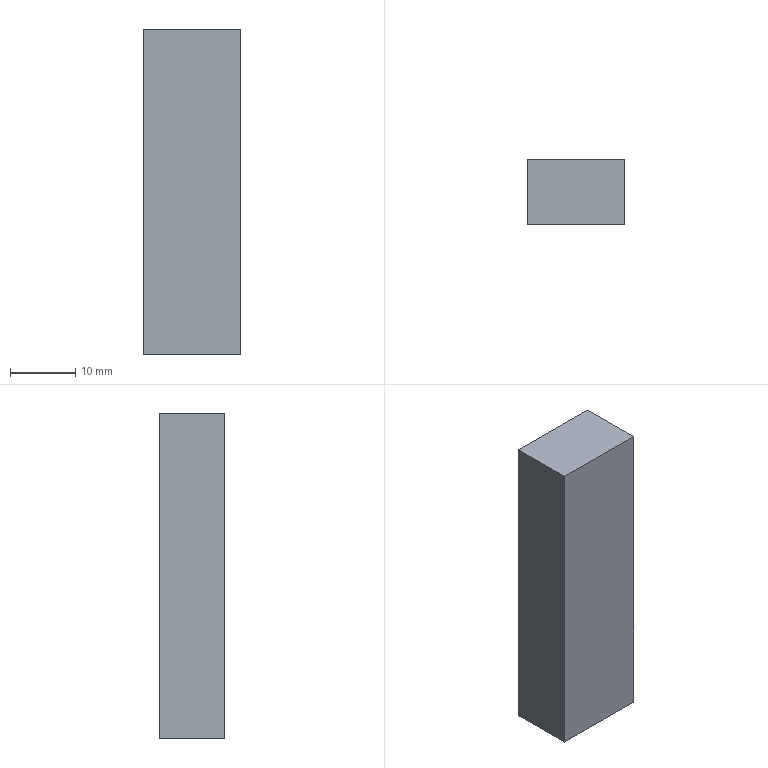Part | NX | features BLOCK 1, DATUM_CSYS 1 | 1 solid | 6 faces | box 15 x 10 x 50 mm | volume 7500 mm3 | plane 6
STEP:
#1=CARTESIAN_POINT('',(15.,0.,50.));
#2=VERTEX_POINT('',#1);
#3=CARTESIAN_POINT('',(0.,0.,50.));
#4=VERTEX_POINT('',#3);
#5=CARTESIAN_POINT('',(7.5,0.,50.));
#6=DIRECTION('',(-1.,0.,0.));
#7=VECTOR('',#6,1000.);
#8=LINE('',#5,#7);
#9=EDGE_CURVE('',#2,#4,#8,.T.);
#10=ORIENTED_EDGE('',*,*,#9,.F.);
#11=CARTESIAN_POINT('',(15.,10.,50.));
#12=VERTEX_POINT('',#11);
#13=CARTESIAN_POINT('',(15.,5.,50.));
#14=DIRECTION('',(0.,-1.,0.));
#15=VECTOR('',#14,1000.);
#16=LINE('',#13,#15);
#17=EDGE_CURVE('',#12,#2,#16,.T.);
#18=ORIENTED_EDGE('',*,*,#17,.F.);
#19=CARTESIAN_POINT('',(0.,10.,50.));
#20=VERTEX_POINT('',#19);
#21=CARTESIAN_POINT('',(7.5,10.,50.));
#22=DIRECTION('',(1.,0.,0.));
#23=VECTOR('',#22,1000.);
#24=LINE('',#21,#23);
#25=EDGE_CURVE('',#20,#12,#24,.T.);
#26=ORIENTED_EDGE('',*,*,#25,.F.);
#27=CARTESIAN_POINT('',(0.,5.,50.));
#28=DIRECTION('',(0.,1.,0.));
#29=VECTOR('',#28,1000.);
#30=LINE('',#27,#29);
#31=EDGE_CURVE('',#4,#20,#30,.T.);
#32=ORIENTED_EDGE('',*,*,#31,.F.);
#33=EDGE_LOOP('',(#10,#18,#26,#32));
#34=FACE_BOUND('',#33,.T.);
#35=CARTESIAN_POINT('',(7.5,5.,50.));
#36=DIRECTION('',(0.,0.,1.));
#37=DIRECTION('',(1.,0.,0.));
#38=AXIS2_PLACEMENT_3D('',#35,#36,#37);
#39=PLANE('',#38);
#40=ADVANCED_FACE('',(#34),#39,.T.);
#41=CARTESIAN_POINT('',(15.,0.,0.));
#42=VERTEX_POINT('',#41);
#43=CARTESIAN_POINT('',(15.,0.,0.));
#44=DIRECTION('',(0.,0.,1.));
#45=VECTOR('',#44,1000.);
#46=LINE('',#43,#45);
#47=EDGE_CURVE('',#42,#2,#46,.T.);
#48=ORIENTED_EDGE('',*,*,#47,.T.);
#49=ORIENTED_EDGE('',*,*,#9,.T.);
#50=CARTESIAN_POINT('',(0.,0.,0.));
#51=VERTEX_POINT('',#50);
#52=CARTESIAN_POINT('',(0.,0.,0.));
#53=DIRECTION('',(0.,0.,1.));
#54=VECTOR('',#53,1000.);
#55=LINE('',#52,#54);
#56=EDGE_CURVE('',#51,#4,#55,.T.);
#57=ORIENTED_EDGE('',*,*,#56,.F.);
#58=CARTESIAN_POINT('',(7.5,0.,0.));
#59=DIRECTION('',(1.,0.,0.));
#60=VECTOR('',#59,1000.);
#61=LINE('',#58,#60);
#62=EDGE_CURVE('',#51,#42,#61,.T.);
#63=ORIENTED_EDGE('',*,*,#62,.T.);
#64=EDGE_LOOP('',(#48,#49,#57,#63));
#65=FACE_BOUND('',#64,.T.);
#66=CARTESIAN_POINT('',(7.5,0.,0.));
#67=DIRECTION('',(0.,-1.,0.));
#68=DIRECTION('',(0.,0.,-1.));
#69=AXIS2_PLACEMENT_3D('',#66,#67,#68);
#70=PLANE('',#69);
#71=ADVANCED_FACE('',(#65),#70,.T.);
#72=ORIENTED_EDGE('',*,*,#56,.T.);
#73=ORIENTED_EDGE('',*,*,#31,.T.);
#74=CARTESIAN_POINT('',(0.,10.,0.));
#75=VERTEX_POINT('',#74);
#76=CARTESIAN_POINT('',(0.,10.,0.));
#77=DIRECTION('',(0.,0.,1.));
#78=VECTOR('',#77,1000.);
#79=LINE('',#76,#78);
#80=EDGE_CURVE('',#75,#20,#79,.T.);
#81=ORIENTED_EDGE('',*,*,#80,.F.);
#82=CARTESIAN_POINT('',(0.,5.,0.));
#83=DIRECTION('',(0.,-1.,0.));
#84=VECTOR('',#83,1000.);
#85=LINE('',#82,#84);
#86=EDGE_CURVE('',#75,#51,#85,.T.);
#87=ORIENTED_EDGE('',*,*,#86,.T.);
#88=EDGE_LOOP('',(#72,#73,#81,#87));
#89=FACE_BOUND('',#88,.T.);
#90=CARTESIAN_POINT('',(0.,5.,0.));
#91=DIRECTION('',(-1.,0.,0.));
#92=DIRECTION('',(0.,0.,1.));
#93=AXIS2_PLACEMENT_3D('',#90,#91,#92);
#94=PLANE('',#93);
#95=ADVANCED_FACE('',(#89),#94,.T.);
#96=ORIENTED_EDGE('',*,*,#80,.T.);
#97=ORIENTED_EDGE('',*,*,#25,.T.);
#98=CARTESIAN_POINT('',(15.,10.,0.));
#99=VERTEX_POINT('',#98);
#100=CARTESIAN_POINT('',(15.,10.,0.));
#101=DIRECTION('',(0.,0.,1.));
#102=VECTOR('',#101,1000.);
#103=LINE('',#100,#102);
#104=EDGE_CURVE('',#99,#12,#103,.T.);
#105=ORIENTED_EDGE('',*,*,#104,.F.);
#106=CARTESIAN_POINT('',(7.5,10.,0.));
#107=DIRECTION('',(-1.,0.,0.));
#108=VECTOR('',#107,1000.);
#109=LINE('',#106,#108);
#110=EDGE_CURVE('',#99,#75,#109,.T.);
#111=ORIENTED_EDGE('',*,*,#110,.T.);
#112=EDGE_LOOP('',(#96,#97,#105,#111));
#113=FACE_BOUND('',#112,.T.);
#114=CARTESIAN_POINT('',(7.5,10.,0.));
#115=DIRECTION('',(0.,1.,0.));
#116=DIRECTION('',(0.,0.,1.));
#117=AXIS2_PLACEMENT_3D('',#114,#115,#116);
#118=PLANE('',#117);
#119=ADVANCED_FACE('',(#113),#118,.T.);
#120=CARTESIAN_POINT('',(15.,5.,0.));
#121=DIRECTION('',(0.,1.,0.));
#122=VECTOR('',#121,1000.);
#123=LINE('',#120,#122);
#124=EDGE_CURVE('',#42,#99,#123,.T.);
#125=ORIENTED_EDGE('',*,*,#124,.F.);
#126=ORIENTED_EDGE('',*,*,#62,.F.);
#127=ORIENTED_EDGE('',*,*,#86,.F.);
#128=ORIENTED_EDGE('',*,*,#110,.F.);
#129=EDGE_LOOP('',(#125,#126,#127,#128));
#130=FACE_BOUND('',#129,.T.);
#131=CARTESIAN_POINT('',(7.5,5.,0.));
#132=DIRECTION('',(0.,0.,-1.));
#133=DIRECTION('',(-1.,0.,0.));
#134=AXIS2_PLACEMENT_3D('',#131,#132,#133);
#135=PLANE('',#134);
#136=ADVANCED_FACE('',(#130),#135,.T.);
#137=ORIENTED_EDGE('',*,*,#124,.T.);
#138=ORIENTED_EDGE('',*,*,#104,.T.);
#139=ORIENTED_EDGE('',*,*,#17,.T.);
#140=ORIENTED_EDGE('',*,*,#47,.F.);
#141=EDGE_LOOP('',(#137,#138,#139,#140));
#142=FACE_BOUND('',#141,.T.);
#143=CARTESIAN_POINT('',(15.,5.,0.));
#144=DIRECTION('',(1.,0.,0.));
#145=DIRECTION('',(0.,0.,-1.));
#146=AXIS2_PLACEMENT_3D('',#143,#144,#145);
#147=PLANE('',#146);
#148=ADVANCED_FACE('',(#142),#147,.T.);
#149=CLOSED_SHELL('',(#40,#71,#95,#119,#136,#148));
#150=MANIFOLD_SOLID_BREP('',#149);
#151=(LENGTH_UNIT()NAMED_UNIT(*)SI_UNIT(.MILLI.,.METRE.));
#152=UNCERTAINTY_MEASURE_WITH_UNIT(LENGTH_MEASURE(0.00001),#151,'','');
#153=(NAMED_UNIT(*)PLANE_ANGLE_UNIT()SI_UNIT($,.RADIAN.));
#154=(NAMED_UNIT(*)SI_UNIT($,.STERADIAN.)SOLID_ANGLE_UNIT());
#155=(GEOMETRIC_REPRESENTATION_CONTEXT(3)GLOBAL_UNCERTAINTY_ASSIGNED_CONTEXT((#152))GLOBAL_UNIT_ASSIGNED_CONTEXT((#151,#153,#154))REPRESENTATION_CONTEXT('',''));
#156=ADVANCED_BREP_SHAPE_REPRESENTATION('',(#150),#155);